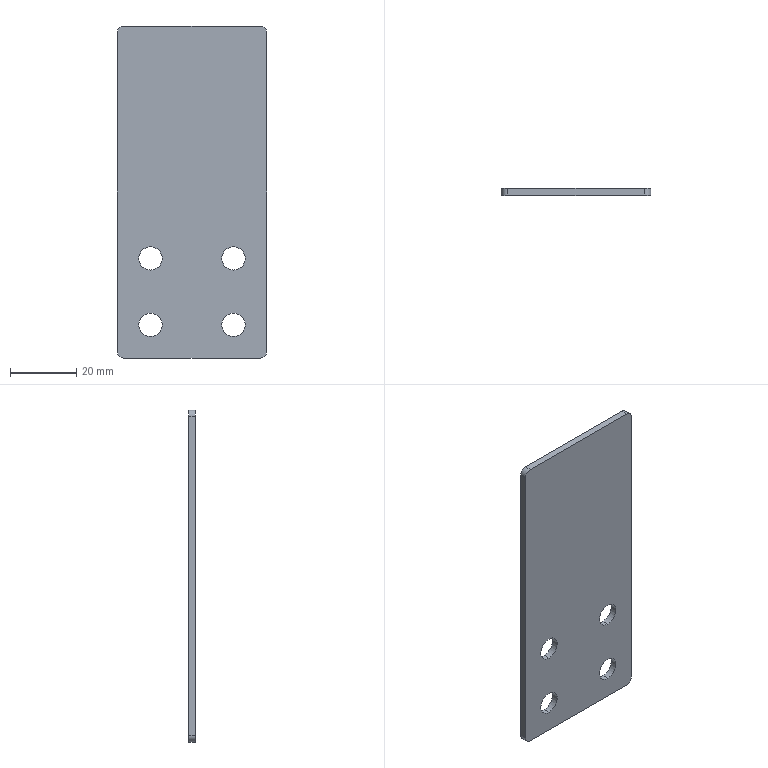Part | STEP file | 1 solid | 18 faces | box 45 x 2 x 100 mm | volume 8685 mm3 | cylinder 12 | plane 6 | commonest cylinder face diameters 7 x8 4 x4